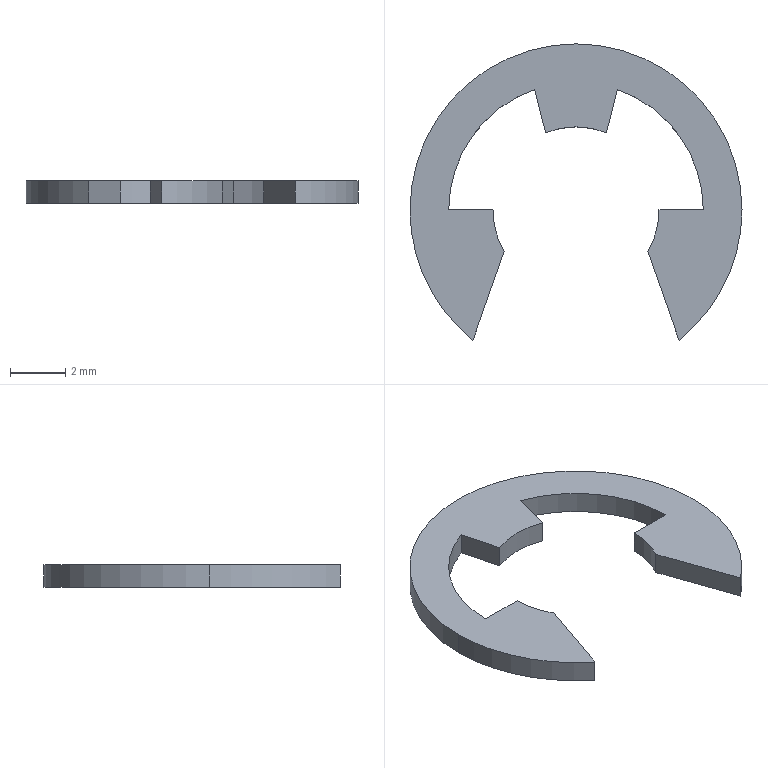Part | STEP file | 0246_016_NETWS6 | 1 solid | 16 faces | box 12 x 10.705 x 0.8 mm | volume 38.915 mm3 | cylinder 8 | plane 8 | commonest cylinder face diameters 6 x3 12 x3 9.2 x2
STEP:
#1=CARTESIAN_POINT('',(0.,0.,0.));
#2=DIRECTION('',(0.,0.,1.));
#3=DIRECTION('',(1.,0.,0.));
#4=AXIS2_PLACEMENT_3D('',#1,#2,#3);
#5=CARTESIAN_POINT('',(6.,0.,-0.4));
#6=VERTEX_POINT('',#5);
#7=CARTESIAN_POINT('',(-6.,0.,-0.4));
#8=VERTEX_POINT('',#7);
#9=CARTESIAN_POINT('',(0.,0.,-0.4));
#10=DIRECTION('',(0.,0.,1.));
#11=DIRECTION('',(1.,0.,0.));
#12=AXIS2_PLACEMENT_3D('',#9,#10,#11);
#13=CIRCLE('',#12,6.);
#14=CARTESIAN_POINT('',(0.,0.,0.4));
#15=DIRECTION('',(0.,0.,1.));
#16=DIRECTION('',(1.,0.,0.));
#17=AXIS2_PLACEMENT_3D('',#14,#15,#16);
#18=CYLINDRICAL_SURFACE('',#17,6.);
#19=CARTESIAN_POINT('',(0.,-0.8));
#20=DIRECTION('',(1.,0.));
#21=VECTOR('',#20,1.);
#22=LINE('',#19,#21);
#23=(GEOMETRIC_REPRESENTATION_CONTEXT(2)PARAMETRIC_REPRESENTATION_CONTEXT()REPRESENTATION_CONTEXT('',''));
#24=DEFINITIONAL_REPRESENTATION('',(#22),#23);
#25=PCURVE('',#18,#24);
#26=CARTESIAN_POINT('',(0.,0.,-0.4));
#27=DIRECTION('',(0.,0.,1.));
#28=DIRECTION('',(1.,0.,0.));
#29=AXIS2_PLACEMENT_3D('',#26,#27,#28);
#30=PLANE('',#29);
#31=CARTESIAN_POINT('',(0.,0.));
#32=DIRECTION('',(1.,0.));
#33=AXIS2_PLACEMENT_2D('',#31,#32);
#34=CIRCLE('',#33,6.);
#35=(GEOMETRIC_REPRESENTATION_CONTEXT(2)PARAMETRIC_REPRESENTATION_CONTEXT()REPRESENTATION_CONTEXT('',''));
#36=DEFINITIONAL_REPRESENTATION('',(#34),#35);
#37=PCURVE('',#30,#36);
#38=SURFACE_CURVE('',#13,(#25,#37),.PCURVE_S1.);
#39=EDGE_CURVE('',#6,#8,#38,.T.);
#40=ORIENTED_EDGE('',*,*,#39,.T.);
#41=CARTESIAN_POINT('',(-6.,0.,0.4));
#42=VERTEX_POINT('',#41);
#43=CARTESIAN_POINT('',(-6.,0.,0.4));
#44=DIRECTION('',(0.,0.,1.));
#45=VECTOR('',#44,1.);
#46=LINE('',#43,#45);
#47=CARTESIAN_POINT('',(3.142,0.));
#48=DIRECTION('',(0.,1.));
#49=VECTOR('',#48,1.);
#50=LINE('',#47,#49);
#51=(GEOMETRIC_REPRESENTATION_CONTEXT(2)PARAMETRIC_REPRESENTATION_CONTEXT()REPRESENTATION_CONTEXT('',''));
#52=DEFINITIONAL_REPRESENTATION('',(#50),#51);
#53=PCURVE('',#18,#52);
#54=CARTESIAN_POINT('',(0.,0.,0.4));
#55=DIRECTION('',(0.,0.,1.));
#56=DIRECTION('',(1.,0.,0.));
#57=AXIS2_PLACEMENT_3D('',#54,#55,#56);
#58=CYLINDRICAL_SURFACE('',#57,6.);
#59=CARTESIAN_POINT('',(3.142,0.));
#60=DIRECTION('',(0.,1.));
#61=VECTOR('',#60,1.);
#62=LINE('',#59,#61);
#63=(GEOMETRIC_REPRESENTATION_CONTEXT(2)PARAMETRIC_REPRESENTATION_CONTEXT()REPRESENTATION_CONTEXT('',''));
#64=DEFINITIONAL_REPRESENTATION('',(#62),#63);
#65=PCURVE('',#58,#64);
#66=SURFACE_CURVE('',#46,(#53,#65),.PCURVE_S1.);
#67=EDGE_CURVE('',#8,#42,#66,.T.);
#68=ORIENTED_EDGE('',*,*,#67,.T.);
#69=CARTESIAN_POINT('',(6.,0.,0.4));
#70=VERTEX_POINT('',#69);
#71=CARTESIAN_POINT('',(0.,0.,0.4));
#72=DIRECTION('',(0.,0.,-1.));
#73=DIRECTION('',(1.,0.,0.));
#74=AXIS2_PLACEMENT_3D('',#71,#72,#73);
#75=CIRCLE('',#74,6.);
#76=CARTESIAN_POINT('',(6.283,0.));
#77=DIRECTION('',(-1.,0.));
#78=VECTOR('',#77,1.);
#79=LINE('',#76,#78);
#80=(GEOMETRIC_REPRESENTATION_CONTEXT(2)PARAMETRIC_REPRESENTATION_CONTEXT()REPRESENTATION_CONTEXT('',''));
#81=DEFINITIONAL_REPRESENTATION('',(#79),#80);
#82=PCURVE('',#18,#81);
#83=CARTESIAN_POINT('',(0.,0.,0.4));
#84=DIRECTION('',(0.,0.,1.));
#85=DIRECTION('',(1.,0.,0.));
#86=AXIS2_PLACEMENT_3D('',#83,#84,#85);
#87=PLANE('',#86);
#88=CARTESIAN_POINT('',(6.,0.));
#89=CARTESIAN_POINT('',(6.,-10.392));
#90=CARTESIAN_POINT('',(-3.,-5.196));
#91=CARTESIAN_POINT('',(-12.,0.));
#92=CARTESIAN_POINT('',(-3.,5.196));
#93=CARTESIAN_POINT('',(6.,10.392));
#94=CARTESIAN_POINT('',(6.,0.));
#95=(BOUNDED_CURVE()B_SPLINE_CURVE(2,(#88,#89,#90,#91,#92,#93,#94),.UNSPECIFIED.,.T.,.F.)B_SPLINE_CURVE_WITH_KNOTS((1,2,2,2,2,1),(-2.094,0.,2.094,4.189,6.283,8.378),.UNSPECIFIED.)CURVE()GEOMETRIC_REPRESENTATION_ITEM()RATIONAL_B_SPLINE_CURVE((1.,0.5,1.,0.5,1.,0.5,1.))REPRESENTATION_ITEM(''));
#96=(GEOMETRIC_REPRESENTATION_CONTEXT(2)PARAMETRIC_REPRESENTATION_CONTEXT()REPRESENTATION_CONTEXT('',''));
#97=DEFINITIONAL_REPRESENTATION('',(#95),#96);
#98=PCURVE('',#87,#97);
#99=SURFACE_CURVE('',#75,(#82,#98),.PCURVE_S1.);
#100=EDGE_CURVE('',#42,#70,#99,.T.);
#101=ORIENTED_EDGE('',*,*,#100,.T.);
#102=CARTESIAN_POINT('',(6.,0.,0.4));
#103=DIRECTION('',(0.,0.,1.));
#104=VECTOR('',#103,1.);
#105=LINE('',#102,#104);
#106=CARTESIAN_POINT('',(0.,0.));
#107=DIRECTION('',(0.,1.));
#108=VECTOR('',#107,1.);
#109=LINE('',#106,#108);
#110=(GEOMETRIC_REPRESENTATION_CONTEXT(2)PARAMETRIC_REPRESENTATION_CONTEXT()REPRESENTATION_CONTEXT('',''));
#111=DEFINITIONAL_REPRESENTATION('',(#109),#110);
#112=PCURVE('',#18,#111);
#113=CARTESIAN_POINT('',(0.,0.,0.4));
#114=DIRECTION('',(0.,0.,1.));
#115=DIRECTION('',(1.,0.,0.));
#116=AXIS2_PLACEMENT_3D('',#113,#114,#115);
#117=CYLINDRICAL_SURFACE('',#116,6.);
#118=CARTESIAN_POINT('',(6.283,0.));
#119=DIRECTION('',(0.,1.));
#120=VECTOR('',#119,1.);
#121=LINE('',#118,#120);
#122=(GEOMETRIC_REPRESENTATION_CONTEXT(2)PARAMETRIC_REPRESENTATION_CONTEXT()REPRESENTATION_CONTEXT('',''));
#123=DEFINITIONAL_REPRESENTATION('',(#121),#122);
#124=PCURVE('',#117,#123);
#125=SURFACE_CURVE('',#105,(#112,#124),.PCURVE_S1.);
#126=EDGE_CURVE('',#6,#70,#125,.T.);
#127=ORIENTED_EDGE('',*,*,#126,.F.);
#128=EDGE_LOOP('',(#40,#68,#101,#127));
#129=FACE_BOUND('',#128,.T.);
#130=ADVANCED_FACE('',(#129),#18,.T.);
#131=CARTESIAN_POINT('',(3.723,-4.705,-0.4));
#132=VERTEX_POINT('',#131);
#133=CARTESIAN_POINT('',(0.,0.,-0.4));
#134=DIRECTION('',(0.,0.,1.));
#135=DIRECTION('',(1.,0.,0.));
#136=AXIS2_PLACEMENT_3D('',#133,#134,#135);
#137=CIRCLE('',#136,6.);
#138=CARTESIAN_POINT('',(0.,-0.8));
#139=DIRECTION('',(1.,0.));
#140=VECTOR('',#139,1.);
#141=LINE('',#138,#140);
#142=(GEOMETRIC_REPRESENTATION_CONTEXT(2)PARAMETRIC_REPRESENTATION_CONTEXT()REPRESENTATION_CONTEXT('',''));
#143=DEFINITIONAL_REPRESENTATION('',(#141),#142);
#144=PCURVE('',#117,#143);
#145=CARTESIAN_POINT('',(0.,0.));
#146=DIRECTION('',(1.,0.));
#147=AXIS2_PLACEMENT_2D('',#145,#146);
#148=CIRCLE('',#147,6.);
#149=(GEOMETRIC_REPRESENTATION_CONTEXT(2)PARAMETRIC_REPRESENTATION_CONTEXT()REPRESENTATION_CONTEXT('',''));
#150=DEFINITIONAL_REPRESENTATION('',(#148),#149);
#151=PCURVE('',#30,#150);
#152=SURFACE_CURVE('',#137,(#144,#151),.PCURVE_S1.);
#153=EDGE_CURVE('',#132,#6,#152,.T.);
#154=ORIENTED_EDGE('',*,*,#153,.T.);
#155=ORIENTED_EDGE('',*,*,#126,.T.);
#156=CARTESIAN_POINT('',(3.723,-4.705,0.4));
#157=VERTEX_POINT('',#156);
#158=CARTESIAN_POINT('',(0.,0.,0.4));
#159=DIRECTION('',(0.,0.,-1.));
#160=DIRECTION('',(1.,0.,0.));
#161=AXIS2_PLACEMENT_3D('',#158,#159,#160);
#162=CIRCLE('',#161,6.);
#163=CARTESIAN_POINT('',(6.283,0.));
#164=DIRECTION('',(-1.,0.));
#165=VECTOR('',#164,1.);
#166=LINE('',#163,#165);
#167=(GEOMETRIC_REPRESENTATION_CONTEXT(2)PARAMETRIC_REPRESENTATION_CONTEXT()REPRESENTATION_CONTEXT('',''));
#168=DEFINITIONAL_REPRESENTATION('',(#166),#167);
#169=PCURVE('',#117,#168);
#170=CARTESIAN_POINT('',(6.,0.));
#171=CARTESIAN_POINT('',(6.,-10.392));
#172=CARTESIAN_POINT('',(-3.,-5.196));
#173=CARTESIAN_POINT('',(-12.,0.));
#174=CARTESIAN_POINT('',(-3.,5.196));
#175=CARTESIAN_POINT('',(6.,10.392));
#176=CARTESIAN_POINT('',(6.,0.));
#177=(BOUNDED_CURVE()B_SPLINE_CURVE(2,(#170,#171,#172,#173,#174,#175,#176),.UNSPECIFIED.,.T.,.F.)B_SPLINE_CURVE_WITH_KNOTS((1,2,2,2,2,1),(-2.094,0.,2.094,4.189,6.283,8.378),.UNSPECIFIED.)CURVE()GEOMETRIC_REPRESENTATION_ITEM()RATIONAL_B_SPLINE_CURVE((1.,0.5,1.,0.5,1.,0.5,1.))REPRESENTATION_ITEM(''));
#178=(GEOMETRIC_REPRESENTATION_CONTEXT(2)PARAMETRIC_REPRESENTATION_CONTEXT()REPRESENTATION_CONTEXT('',''));
#179=DEFINITIONAL_REPRESENTATION('',(#177),#178);
#180=PCURVE('',#87,#179);
#181=SURFACE_CURVE('',#162,(#169,#180),.PCURVE_S1.);
#182=EDGE_CURVE('',#70,#157,#181,.T.);
#183=ORIENTED_EDGE('',*,*,#182,.T.);
#184=CARTESIAN_POINT('',(3.723,-4.705,0.4));
#185=DIRECTION('',(0.,0.,-1.));
#186=VECTOR('',#185,1.);
#187=LINE('',#184,#186);
#188=CARTESIAN_POINT('',(5.382,0.));
#189=DIRECTION('',(0.,-1.));
#190=VECTOR('',#189,1.);
#191=LINE('',#188,#190);
#192=(GEOMETRIC_REPRESENTATION_CONTEXT(2)PARAMETRIC_REPRESENTATION_CONTEXT()REPRESENTATION_CONTEXT('',''));
#193=DEFINITIONAL_REPRESENTATION('',(#191),#192);
#194=PCURVE('',#117,#193);
#195=CARTESIAN_POINT('',(2.6,-1.497,0.4));
#196=DIRECTION('',(-0.9438,-0.3305,0.));
#197=DIRECTION('',(0.3305,-0.9438,0.));
#198=AXIS2_PLACEMENT_3D('',#195,#196,#197);
#199=PLANE('',#198);
#200=CARTESIAN_POINT('',(3.399,0.));
#201=DIRECTION('',(0.,-1.));
#202=VECTOR('',#201,1.);
#203=LINE('',#200,#202);
#204=(GEOMETRIC_REPRESENTATION_CONTEXT(2)PARAMETRIC_REPRESENTATION_CONTEXT()REPRESENTATION_CONTEXT('',''));
#205=DEFINITIONAL_REPRESENTATION('',(#203),#204);
#206=PCURVE('',#199,#205);
#207=SURFACE_CURVE('',#187,(#194,#206),.PCURVE_S1.);
#208=EDGE_CURVE('',#157,#132,#207,.T.);
#209=ORIENTED_EDGE('',*,*,#208,.T.);
#210=EDGE_LOOP('',(#154,#155,#183,#209));
#211=FACE_BOUND('',#210,.T.);
#212=ADVANCED_FACE('',(#211),#117,.T.);
#213=CARTESIAN_POINT('',(-3.723,-4.705,-0.4));
#214=VERTEX_POINT('',#213);
#215=CARTESIAN_POINT('',(-2.6,-1.497,-0.4));
#216=VERTEX_POINT('',#215);
#217=CARTESIAN_POINT('',(-3.723,-4.705,-0.4));
#218=DIRECTION('',(0.3305,0.9438,0.));
#219=VECTOR('',#218,1.);
#220=LINE('',#217,#219);
#221=CARTESIAN_POINT('',(-3.723,-4.705));
#222=DIRECTION('',(0.3305,0.9438));
#223=VECTOR('',#222,1.);
#224=LINE('',#221,#223);
#225=(GEOMETRIC_REPRESENTATION_CONTEXT(2)PARAMETRIC_REPRESENTATION_CONTEXT()REPRESENTATION_CONTEXT('',''));
#226=DEFINITIONAL_REPRESENTATION('',(#224),#225);
#227=PCURVE('',#30,#226);
#228=CARTESIAN_POINT('',(-3.723,-4.705,0.4));
#229=DIRECTION('',(0.9438,-0.3305,0.));
#230=DIRECTION('',(0.3305,0.9438,0.));
#231=AXIS2_PLACEMENT_3D('',#228,#229,#230);
#232=PLANE('',#231);
#233=CARTESIAN_POINT('',(0.,-0.8));
#234=DIRECTION('',(1.,0.));
#235=VECTOR('',#234,1.);
#236=LINE('',#233,#235);
#237=(GEOMETRIC_REPRESENTATION_CONTEXT(2)PARAMETRIC_REPRESENTATION_CONTEXT()REPRESENTATION_CONTEXT('',''));
#238=DEFINITIONAL_REPRESENTATION('',(#236),#237);
#239=PCURVE('',#232,#238);
#240=SURFACE_CURVE('',#220,(#227,#239),.PCURVE_S1.);
#241=EDGE_CURVE('',#214,#216,#240,.T.);
#242=ORIENTED_EDGE('',*,*,#241,.F.);
#243=CARTESIAN_POINT('',(0.,0.,-0.4));
#244=DIRECTION('',(0.,0.,1.));
#245=DIRECTION('',(1.,0.,0.));
#246=AXIS2_PLACEMENT_3D('',#243,#244,#245);
#247=CIRCLE('',#246,6.);
#248=CARTESIAN_POINT('',(0.,0.));
#249=DIRECTION('',(1.,0.));
#250=AXIS2_PLACEMENT_2D('',#248,#249);
#251=CIRCLE('',#250,6.);
#252=(GEOMETRIC_REPRESENTATION_CONTEXT(2)PARAMETRIC_REPRESENTATION_CONTEXT()REPRESENTATION_CONTEXT('',''));
#253=DEFINITIONAL_REPRESENTATION('',(#251),#252);
#254=PCURVE('',#30,#253);
#255=CARTESIAN_POINT('',(0.,-0.8));
#256=DIRECTION('',(1.,0.));
#257=VECTOR('',#256,1.);
#258=LINE('',#255,#257);
#259=(GEOMETRIC_REPRESENTATION_CONTEXT(2)PARAMETRIC_REPRESENTATION_CONTEXT()REPRESENTATION_CONTEXT('',''));
#260=DEFINITIONAL_REPRESENTATION('',(#258),#259);
#261=PCURVE('',#58,#260);
#262=SURFACE_CURVE('',#247,(#254,#261),.PCURVE_S1.);
#263=EDGE_CURVE('',#8,#214,#262,.T.);
#264=ORIENTED_EDGE('',*,*,#263,.F.);
#265=ORIENTED_EDGE('',*,*,#39,.F.);
#266=ORIENTED_EDGE('',*,*,#153,.F.);
#267=CARTESIAN_POINT('',(2.6,-1.497,-0.4));
#268=VERTEX_POINT('',#267);
#269=CARTESIAN_POINT('',(2.6,-1.497,-0.4));
#270=DIRECTION('',(0.3305,-0.9438,0.));
#271=VECTOR('',#270,1.);
#272=LINE('',#269,#271);
#273=CARTESIAN_POINT('',(2.6,-1.497));
#274=DIRECTION('',(0.3305,-0.9438));
#275=VECTOR('',#274,1.);
#276=LINE('',#273,#275);
#277=(GEOMETRIC_REPRESENTATION_CONTEXT(2)PARAMETRIC_REPRESENTATION_CONTEXT()REPRESENTATION_CONTEXT('',''));
#278=DEFINITIONAL_REPRESENTATION('',(#276),#277);
#279=PCURVE('',#30,#278);
#280=CARTESIAN_POINT('',(0.,-0.8));
#281=DIRECTION('',(1.,0.));
#282=VECTOR('',#281,1.);
#283=LINE('',#280,#282);
#284=(GEOMETRIC_REPRESENTATION_CONTEXT(2)PARAMETRIC_REPRESENTATION_CONTEXT()REPRESENTATION_CONTEXT('',''));
#285=DEFINITIONAL_REPRESENTATION('',(#283),#284);
#286=PCURVE('',#199,#285);
#287=SURFACE_CURVE('',#272,(#279,#286),.PCURVE_S1.);
#288=EDGE_CURVE('',#268,#132,#287,.T.);
#289=ORIENTED_EDGE('',*,*,#288,.F.);
#290=CARTESIAN_POINT('',(3.,0.,-0.4));
#291=VERTEX_POINT('',#290);
#292=CARTESIAN_POINT('',(0.,0.,-0.4));
#293=DIRECTION('',(0.,0.,-1.));
#294=DIRECTION('',(1.,0.,0.));
#295=AXIS2_PLACEMENT_3D('',#292,#293,#294);
#296=CIRCLE('',#295,3.);
#297=CARTESIAN_POINT('',(3.,0.));
#298=CARTESIAN_POINT('',(3.,-5.196));
#299=CARTESIAN_POINT('',(-1.5,-2.598));
#300=CARTESIAN_POINT('',(-6.,0.));
#301=CARTESIAN_POINT('',(-1.5,2.598));
#302=CARTESIAN_POINT('',(3.,5.196));
#303=CARTESIAN_POINT('',(3.,0.));
#304=(BOUNDED_CURVE()B_SPLINE_CURVE(2,(#297,#298,#299,#300,#301,#302,#303),.UNSPECIFIED.,.T.,.F.)B_SPLINE_CURVE_WITH_KNOTS((1,2,2,2,2,1),(-2.094,0.,2.094,4.189,6.283,8.378),.UNSPECIFIED.)CURVE()GEOMETRIC_REPRESENTATION_ITEM()RATIONAL_B_SPLINE_CURVE((1.,0.5,1.,0.5,1.,0.5,1.))REPRESENTATION_ITEM(''));
#305=(GEOMETRIC_REPRESENTATION_CONTEXT(2)PARAMETRIC_REPRESENTATION_CONTEXT()REPRESENTATION_CONTEXT('',''));
#306=DEFINITIONAL_REPRESENTATION('',(#304),#305);
#307=PCURVE('',#30,#306);
#308=CARTESIAN_POINT('',(0.,0.,0.4));
#309=DIRECTION('',(0.,0.,1.));
#310=DIRECTION('',(1.,0.,0.));
#311=AXIS2_PLACEMENT_3D('',#308,#309,#310);
#312=CYLINDRICAL_SURFACE('',#311,3.);
#313=CARTESIAN_POINT('',(6.283,-0.8));
#314=DIRECTION('',(-1.,0.));
#315=VECTOR('',#314,1.);
#316=LINE('',#313,#315);
#317=(GEOMETRIC_REPRESENTATION_CONTEXT(2)PARAMETRIC_REPRESENTATION_CONTEXT()REPRESENTATION_CONTEXT('',''));
#318=DEFINITIONAL_REPRESENTATION('',(#316),#317);
#319=PCURVE('',#312,#318);
#320=SURFACE_CURVE('',#296,(#307,#319),.PCURVE_S1.);
#321=EDGE_CURVE('',#291,#268,#320,.T.);
#322=ORIENTED_EDGE('',*,*,#321,.F.);
#323=CARTESIAN_POINT('',(4.6,0.,-0.4));
#324=VERTEX_POINT('',#323);
#325=CARTESIAN_POINT('',(0.,0.,-0.4));
#326=DIRECTION('',(-1.,0.,0.));
#327=VECTOR('',#326,1.);
#328=LINE('',#325,#327);
#329=CARTESIAN_POINT('',(0.,0.));
#330=DIRECTION('',(-1.,0.));
#331=VECTOR('',#330,1.);
#332=LINE('',#329,#331);
#333=(GEOMETRIC_REPRESENTATION_CONTEXT(2)PARAMETRIC_REPRESENTATION_CONTEXT()REPRESENTATION_CONTEXT('',''));
#334=DEFINITIONAL_REPRESENTATION('',(#332),#333);
#335=PCURVE('',#30,#334);
#336=CARTESIAN_POINT('',(4.6,0.,0.4));
#337=DIRECTION('',(0.,1.,0.));
#338=DIRECTION('',(0.,0.,1.));
#339=AXIS2_PLACEMENT_3D('',#336,#337,#338);
#340=PLANE('',#339);
#341=CARTESIAN_POINT('',(-0.8,-4.6));
#342=DIRECTION('',(0.,-1.));
#343=VECTOR('',#342,1.);
#344=LINE('',#341,#343);
#345=(GEOMETRIC_REPRESENTATION_CONTEXT(2)PARAMETRIC_REPRESENTATION_CONTEXT()REPRESENTATION_CONTEXT('',''));
#346=DEFINITIONAL_REPRESENTATION('',(#344),#345);
#347=PCURVE('',#340,#346);
#348=SURFACE_CURVE('',#328,(#335,#347),.PCURVE_S1.);
#349=EDGE_CURVE('',#324,#291,#348,.T.);
#350=ORIENTED_EDGE('',*,*,#349,.F.);
#351=CARTESIAN_POINT('',(1.5,4.349,-0.4));
#352=VERTEX_POINT('',#351);
#353=CARTESIAN_POINT('',(0.,0.,-0.4));
#354=DIRECTION('',(0.,0.,-1.));
#355=DIRECTION('',(1.,0.,0.));
#356=AXIS2_PLACEMENT_3D('',#353,#354,#355);
#357=CIRCLE('',#356,4.6);
#358=CARTESIAN_POINT('',(4.6,0.));
#359=CARTESIAN_POINT('',(4.6,-7.967));
#360=CARTESIAN_POINT('',(-2.3,-3.984));
#361=CARTESIAN_POINT('',(-9.2,0.));
#362=CARTESIAN_POINT('',(-2.3,3.984));
#363=CARTESIAN_POINT('',(4.6,7.967));
#364=CARTESIAN_POINT('',(4.6,0.));
#365=(BOUNDED_CURVE()B_SPLINE_CURVE(2,(#358,#359,#360,#361,#362,#363,#364),.UNSPECIFIED.,.T.,.F.)B_SPLINE_CURVE_WITH_KNOTS((1,2,2,2,2,1),(-2.094,0.,2.094,4.189,6.283,8.378),.UNSPECIFIED.)CURVE()GEOMETRIC_REPRESENTATION_ITEM()RATIONAL_B_SPLINE_CURVE((1.,0.5,1.,0.5,1.,0.5,1.))REPRESENTATION_ITEM(''));
#366=(GEOMETRIC_REPRESENTATION_CONTEXT(2)PARAMETRIC_REPRESENTATION_CONTEXT()REPRESENTATION_CONTEXT('',''));
#367=DEFINITIONAL_REPRESENTATION('',(#365),#366);
#368=PCURVE('',#30,#367);
#369=CARTESIAN_POINT('',(0.,0.,0.4));
#370=DIRECTION('',(0.,0.,1.));
#371=DIRECTION('',(1.,0.,0.));
#372=AXIS2_PLACEMENT_3D('',#369,#370,#371);
#373=CYLINDRICAL_SURFACE('',#372,4.6);
#374=CARTESIAN_POINT('',(6.283,-0.8));
#375=DIRECTION('',(-1.,0.));
#376=VECTOR('',#375,1.);
#377=LINE('',#374,#376);
#378=(GEOMETRIC_REPRESENTATION_CONTEXT(2)PARAMETRIC_REPRESENTATION_CONTEXT()REPRESENTATION_CONTEXT('',''));
#379=DEFINITIONAL_REPRESENTATION('',(#377),#378);
#380=PCURVE('',#373,#379);
#381=SURFACE_CURVE('',#357,(#368,#380),.PCURVE_S1.);
#382=EDGE_CURVE('',#352,#324,#381,.T.);
#383=ORIENTED_EDGE('',*,*,#382,.F.);
#384=CARTESIAN_POINT('',(1.1,2.791,-0.4));
#385=VERTEX_POINT('',#384);
#386=CARTESIAN_POINT('',(1.1,2.791,-0.4));
#387=DIRECTION('',(0.2487,0.9686,0.));
#388=VECTOR('',#387,1.);
#389=LINE('',#386,#388);
#390=CARTESIAN_POINT('',(1.1,2.791));
#391=DIRECTION('',(0.2487,0.9686));
#392=VECTOR('',#391,1.);
#393=LINE('',#390,#392);
#394=(GEOMETRIC_REPRESENTATION_CONTEXT(2)PARAMETRIC_REPRESENTATION_CONTEXT()REPRESENTATION_CONTEXT('',''));
#395=DEFINITIONAL_REPRESENTATION('',(#393),#394);
#396=PCURVE('',#30,#395);
#397=CARTESIAN_POINT('',(1.1,2.791,0.4));
#398=DIRECTION('',(0.9686,-0.2487,0.));
#399=DIRECTION('',(0.2487,0.9686,0.));
#400=AXIS2_PLACEMENT_3D('',#397,#398,#399);
#401=PLANE('',#400);
#402=CARTESIAN_POINT('',(0.,-0.8));
#403=DIRECTION('',(1.,0.));
#404=VECTOR('',#403,1.);
#405=LINE('',#402,#404);
#406=(GEOMETRIC_REPRESENTATION_CONTEXT(2)PARAMETRIC_REPRESENTATION_CONTEXT()REPRESENTATION_CONTEXT('',''));
#407=DEFINITIONAL_REPRESENTATION('',(#405),#406);
#408=PCURVE('',#401,#407);
#409=SURFACE_CURVE('',#389,(#396,#408),.PCURVE_S1.);
#410=EDGE_CURVE('',#385,#352,#409,.T.);
#411=ORIENTED_EDGE('',*,*,#410,.F.);
#412=CARTESIAN_POINT('',(-1.1,2.791,-0.4));
#413=VERTEX_POINT('',#412);
#414=CARTESIAN_POINT('',(0.,0.,-0.4));
#415=DIRECTION('',(0.,0.,-1.));
#416=DIRECTION('',(1.,0.,0.));
#417=AXIS2_PLACEMENT_3D('',#414,#415,#416);
#418=CIRCLE('',#417,3.);
#419=CARTESIAN_POINT('',(3.,0.));
#420=CARTESIAN_POINT('',(3.,-5.196));
#421=CARTESIAN_POINT('',(-1.5,-2.598));
#422=CARTESIAN_POINT('',(-6.,0.));
#423=CARTESIAN_POINT('',(-1.5,2.598));
#424=CARTESIAN_POINT('',(3.,5.196));
#425=CARTESIAN_POINT('',(3.,0.));
#426=(BOUNDED_CURVE()B_SPLINE_CURVE(2,(#419,#420,#421,#422,#423,#424,#425),.UNSPECIFIED.,.T.,.F.)B_SPLINE_CURVE_WITH_KNOTS((1,2,2,2,2,1),(-2.094,0.,2.094,4.189,6.283,8.378),.UNSPECIFIED.)CURVE()GEOMETRIC_REPRESENTATION_ITEM()RATIONAL_B_SPLINE_CURVE((1.,0.5,1.,0.5,1.,0.5,1.))REPRESENTATION_ITEM(''));
#427=(GEOMETRIC_REPRESENTATION_CONTEXT(2)PARAMETRIC_REPRESENTATION_CONTEXT()REPRESENTATION_CONTEXT('',''));
#428=DEFINITIONAL_REPRESENTATION('',(#426),#427);
#429=PCURVE('',#30,#428);
#430=CARTESIAN_POINT('',(0.,0.,0.4));
#431=DIRECTION('',(0.,0.,1.));
#432=DIRECTION('',(1.,0.,0.));
#433=AXIS2_PLACEMENT_3D('',#430,#431,#432);
#434=CYLINDRICAL_SURFACE('',#433,3.);
#435=CARTESIAN_POINT('',(6.283,-0.8));
#436=DIRECTION('',(-1.,0.));
#437=VECTOR('',#436,1.);
#438=LINE('',#435,#437);
#439=(GEOMETRIC_REPRESENTATION_CONTEXT(2)PARAMETRIC_REPRESENTATION_CONTEXT()REPRESENTATION_CONTEXT('',''));
#440=DEFINITIONAL_REPRESENTATION('',(#438),#439);
#441=PCURVE('',#434,#440);
#442=SURFACE_CURVE('',#418,(#429,#441),.PCURVE_S1.);
#443=EDGE_CURVE('',#413,#385,#442,.T.);
#444=ORIENTED_EDGE('',*,*,#443,.F.);
#445=CARTESIAN_POINT('',(-1.5,4.349,-0.4));
#446=VERTEX_POINT('',#445);
#447=CARTESIAN_POINT('',(-1.5,4.349,-0.4));
#448=DIRECTION('',(0.2487,-0.9686,0.));
#449=VECTOR('',#448,1.);
#450=LINE('',#447,#449);
#451=CARTESIAN_POINT('',(-1.5,4.349));
#452=DIRECTION('',(0.2487,-0.9686));
#453=VECTOR('',#452,1.);
#454=LINE('',#451,#453);
#455=(GEOMETRIC_REPRESENTATION_CONTEXT(2)PARAMETRIC_REPRESENTATION_CONTEXT()REPRESENTATION_CONTEXT('',''));
#456=DEFINITIONAL_REPRESENTATION('',(#454),#455);
#457=PCURVE('',#30,#456);
#458=CARTESIAN_POINT('',(-1.5,4.349,0.4));
#459=DIRECTION('',(-0.9686,-0.2487,0.));
#460=DIRECTION('',(0.2487,-0.9686,0.));
#461=AXIS2_PLACEMENT_3D('',#458,#459,#460);
#462=PLANE('',#461);
#463=CARTESIAN_POINT('',(0.,-0.8));
#464=DIRECTION('',(1.,0.));
#465=VECTOR('',#464,1.);
#466=LINE('',#463,#465);
#467=(GEOMETRIC_REPRESENTATION_CONTEXT(2)PARAMETRIC_REPRESENTATION_CONTEXT()REPRESENTATION_CONTEXT('',''));
#468=DEFINITIONAL_REPRESENTATION('',(#466),#467);
#469=PCURVE('',#462,#468);
#470=SURFACE_CURVE('',#450,(#457,#469),.PCURVE_S1.);
#471=EDGE_CURVE('',#446,#413,#470,.T.);
#472=ORIENTED_EDGE('',*,*,#471,.F.);
#473=CARTESIAN_POINT('',(-4.6,0.,-0.4));
#474=VERTEX_POINT('',#473);
#475=CARTESIAN_POINT('',(0.,0.,-0.4));
#476=DIRECTION('',(0.,0.,-1.));
#477=DIRECTION('',(1.,0.,0.));
#478=AXIS2_PLACEMENT_3D('',#475,#476,#477);
#479=CIRCLE('',#478,4.6);
#480=CARTESIAN_POINT('',(4.6,0.));
#481=CARTESIAN_POINT('',(4.6,-7.967));
#482=CARTESIAN_POINT('',(-2.3,-3.984));
#483=CARTESIAN_POINT('',(-9.2,0.));
#484=CARTESIAN_POINT('',(-2.3,3.984));
#485=CARTESIAN_POINT('',(4.6,7.967));
#486=CARTESIAN_POINT('',(4.6,0.));
#487=(BOUNDED_CURVE()B_SPLINE_CURVE(2,(#480,#481,#482,#483,#484,#485,#486),.UNSPECIFIED.,.T.,.F.)B_SPLINE_CURVE_WITH_KNOTS((1,2,2,2,2,1),(-2.094,0.,2.094,4.189,6.283,8.378),.UNSPECIFIED.)CURVE()GEOMETRIC_REPRESENTATION_ITEM()RATIONAL_B_SPLINE_CURVE((1.,0.5,1.,0.5,1.,0.5,1.))REPRESENTATION_ITEM(''));
#488=(GEOMETRIC_REPRESENTATION_CONTEXT(2)PARAMETRIC_REPRESENTATION_CONTEXT()REPRESENTATION_CONTEXT('',''));
#489=DEFINITIONAL_REPRESENTATION('',(#487),#488);
#490=PCURVE('',#30,#489);
#491=CARTESIAN_POINT('',(0.,0.,0.4));
#492=DIRECTION('',(0.,0.,1.));
#493=DIRECTION('',(1.,0.,0.));
#494=AXIS2_PLACEMENT_3D('',#491,#492,#493);
#495=CYLINDRICAL_SURFACE('',#494,4.6);
#496=CARTESIAN_POINT('',(6.283,-0.8));
#497=DIRECTION('',(-1.,0.));
#498=VECTOR('',#497,1.);
#499=LINE('',#496,#498);
#500=(GEOMETRIC_REPRESENTATION_CONTEXT(2)PARAMETRIC_REPRESENTATION_CONTEXT()REPRESENTATION_CONTEXT('',''));
#501=DEFINITIONAL_REPRESENTATION('',(#499),#500);
#502=PCURVE('',#495,#501);
#503=SURFACE_CURVE('',#479,(#490,#502),.PCURVE_S1.);
#504=EDGE_CURVE('',#474,#446,#503,.T.);
#505=ORIENTED_EDGE('',*,*,#504,.F.);
#506=CARTESIAN_POINT('',(-3.,0.,-0.4));
#507=VERTEX_POINT('',#506);
#508=CARTESIAN_POINT('',(0.,0.,-0.4));
#509=DIRECTION('',(-1.,0.,0.));
#510=VECTOR('',#509,1.);
#511=LINE('',#508,#510);
#512=CARTESIAN_POINT('',(0.,0.));
#513=DIRECTION('',(-1.,0.));
#514=VECTOR('',#513,1.);
#515=LINE('',#512,#514);
#516=(GEOMETRIC_REPRESENTATION_CONTEXT(2)PARAMETRIC_REPRESENTATION_CONTEXT()REPRESENTATION_CONTEXT('',''));
#517=DEFINITIONAL_REPRESENTATION('',(#515),#516);
#518=PCURVE('',#30,#517);
#519=CARTESIAN_POINT('',(-3.,0.,0.4));
#520=DIRECTION('',(0.,1.,0.));
#521=DIRECTION('',(0.,0.,1.));
#522=AXIS2_PLACEMENT_3D('',#519,#520,#521);
#523=PLANE('',#522);
#524=CARTESIAN_POINT('',(-0.8,3.));
#525=DIRECTION('',(0.,-1.));
#526=VECTOR('',#525,1.);
#527=LINE('',#524,#526);
#528=(GEOMETRIC_REPRESENTATION_CONTEXT(2)PARAMETRIC_REPRESENTATION_CONTEXT()REPRESENTATION_CONTEXT('',''));
#529=DEFINITIONAL_REPRESENTATION('',(#527),#528);
#530=PCURVE('',#523,#529);
#531=SURFACE_CURVE('',#511,(#518,#530),.PCURVE_S1.);
#532=EDGE_CURVE('',#507,#474,#531,.T.);
#533=ORIENTED_EDGE('',*,*,#532,.F.);
#534=CARTESIAN_POINT('',(0.,0.,-0.4));
#535=DIRECTION('',(0.,0.,-1.));
#536=DIRECTION('',(1.,0.,0.));
#537=AXIS2_PLACEMENT_3D('',#534,#535,#536);
#538=CIRCLE('',#537,3.);
#539=CARTESIAN_POINT('',(3.,0.));
#540=CARTESIAN_POINT('',(3.,-5.196));
#541=CARTESIAN_POINT('',(-1.5,-2.598));
#542=CARTESIAN_POINT('',(-6.,0.));
#543=CARTESIAN_POINT('',(-1.5,2.598));
#544=CARTESIAN_POINT('',(3.,5.196));
#545=CARTESIAN_POINT('',(3.,0.));
#546=(BOUNDED_CURVE()B_SPLINE_CURVE(2,(#539,#540,#541,#542,#543,#544,#545),.UNSPECIFIED.,.T.,.F.)B_SPLINE_CURVE_WITH_KNOTS((1,2,2,2,2,1),(-2.094,0.,2.094,4.189,6.283,8.378),.UNSPECIFIED.)CURVE()GEOMETRIC_REPRESENTATION_ITEM()RATIONAL_B_SPLINE_CURVE((1.,0.5,1.,0.5,1.,0.5,1.))REPRESENTATION_ITEM(''));
#547=(GEOMETRIC_REPRESENTATION_CONTEXT(2)PARAMETRIC_REPRESENTATION_CONTEXT()REPRESENTATION_CONTEXT('',''));
#548=DEFINITIONAL_REPRESENTATION('',(#546),#547);
#549=PCURVE('',#30,#548);
#550=CARTESIAN_POINT('',(0.,0.,0.4));
#551=DIRECTION('',(0.,0.,1.));
#552=DIRECTION('',(1.,0.,0.));
#553=AXIS2_PLACEMENT_3D('',#550,#551,#552);
#554=CYLINDRICAL_SURFACE('',#553,3.);
#555=CARTESIAN_POINT('',(6.283,-0.8));
#556=DIRECTION('',(-1.,0.));
#557=VECTOR('',#556,1.);
#558=LINE('',#555,#557);
#559=(GEOMETRIC_REPRESENTATION_CONTEXT(2)PARAMETRIC_REPRESENTATION_CONTEXT()REPRESENTATION_CONTEXT('',''));
#560=DEFINITIONAL_REPRESENTATION('',(#558),#559);
#561=PCURVE('',#554,#560);
#562=SURFACE_CURVE('',#538,(#549,#561),.PCURVE_S1.);
#563=EDGE_CURVE('',#216,#507,#562,.T.);
#564=ORIENTED_EDGE('',*,*,#563,.F.);
#565=EDGE_LOOP('',(#242,#264,#265,#266,#289,#322,#350,#383,#411,#444,#472,#505,#533,#564));
#566=FACE_BOUND('',#565,.T.);
#567=ADVANCED_FACE('',(#566),#30,.F.);
#568=CARTESIAN_POINT('',(-2.6,-1.497,0.4));
#569=VERTEX_POINT('',#568);
#570=CARTESIAN_POINT('',(-3.723,-4.705,0.4));
#571=VERTEX_POINT('',#570);
#572=CARTESIAN_POINT('',(-3.723,-4.705,0.4));
#573=DIRECTION('',(-0.3305,-0.9438,0.));
#574=VECTOR('',#573,1.);
#575=LINE('',#572,#574);
#576=CARTESIAN_POINT('',(0.,0.));
#577=DIRECTION('',(-1.,0.));
#578=VECTOR('',#577,1.);
#579=LINE('',#576,#578);
#580=(GEOMETRIC_REPRESENTATION_CONTEXT(2)PARAMETRIC_REPRESENTATION_CONTEXT()REPRESENTATION_CONTEXT('',''));
#581=DEFINITIONAL_REPRESENTATION('',(#579),#580);
#582=PCURVE('',#232,#581);
#583=CARTESIAN_POINT('',(-3.723,-4.705));
#584=DIRECTION('',(-0.3305,-0.9438));
#585=VECTOR('',#584,1.);
#586=LINE('',#583,#585);
#587=(GEOMETRIC_REPRESENTATION_CONTEXT(2)PARAMETRIC_REPRESENTATION_CONTEXT()REPRESENTATION_CONTEXT('',''));
#588=DEFINITIONAL_REPRESENTATION('',(#586),#587);
#589=PCURVE('',#87,#588);
#590=SURFACE_CURVE('',#575,(#582,#589),.PCURVE_S1.);
#591=EDGE_CURVE('',#569,#571,#590,.T.);
#592=ORIENTED_EDGE('',*,*,#591,.T.);
#593=CARTESIAN_POINT('',(-3.723,-4.705,0.4));
#594=DIRECTION('',(0.,0.,-1.));
#595=VECTOR('',#594,1.);
#596=LINE('',#593,#595);
#597=CARTESIAN_POINT('',(0.,0.));
#598=DIRECTION('',(0.,-1.));
#599=VECTOR('',#598,1.);
#600=LINE('',#597,#599);
#601=(GEOMETRIC_REPRESENTATION_CONTEXT(2)PARAMETRIC_REPRESENTATION_CONTEXT()REPRESENTATION_CONTEXT('',''));
#602=DEFINITIONAL_REPRESENTATION('',(#600),#601);
#603=PCURVE('',#232,#602);
#604=CARTESIAN_POINT('',(4.043,0.));
#605=DIRECTION('',(0.,-1.));
#606=VECTOR('',#605,1.);
#607=LINE('',#604,#606);
#608=(GEOMETRIC_REPRESENTATION_CONTEXT(2)PARAMETRIC_REPRESENTATION_CONTEXT()REPRESENTATION_CONTEXT('',''));
#609=DEFINITIONAL_REPRESENTATION('',(#607),#608);
#610=PCURVE('',#58,#609);
#611=SURFACE_CURVE('',#596,(#603,#610),.PCURVE_S1.);
#612=EDGE_CURVE('',#571,#214,#611,.T.);
#613=ORIENTED_EDGE('',*,*,#612,.T.);
#614=ORIENTED_EDGE('',*,*,#241,.T.);
#615=CARTESIAN_POINT('',(-2.6,-1.497,0.4));
#616=DIRECTION('',(0.,0.,1.));
#617=VECTOR('',#616,1.);
#618=LINE('',#615,#617);
#619=CARTESIAN_POINT('',(3.399,0.));
#620=DIRECTION('',(0.,1.));
#621=VECTOR('',#620,1.);
#622=LINE('',#619,#621);
#623=(GEOMETRIC_REPRESENTATION_CONTEXT(2)PARAMETRIC_REPRESENTATION_CONTEXT()REPRESENTATION_CONTEXT('',''));
#624=DEFINITIONAL_REPRESENTATION('',(#622),#623);
#625=PCURVE('',#232,#624);
#626=CARTESIAN_POINT('',(3.664,0.));
#627=DIRECTION('',(0.,1.));
#628=VECTOR('',#627,1.);
#629=LINE('',#626,#628);
#630=(GEOMETRIC_REPRESENTATION_CONTEXT(2)PARAMETRIC_REPRESENTATION_CONTEXT()REPRESENTATION_CONTEXT('',''));
#631=DEFINITIONAL_REPRESENTATION('',(#629),#630);
#632=PCURVE('',#554,#631);
#633=SURFACE_CURVE('',#618,(#625,#632),.PCURVE_S1.);
#634=EDGE_CURVE('',#216,#569,#633,.T.);
#635=ORIENTED_EDGE('',*,*,#634,.T.);
#636=EDGE_LOOP('',(#592,#613,#614,#635));
#637=FACE_BOUND('',#636,.T.);
#638=ADVANCED_FACE('',(#637),#232,.T.);
#639=ORIENTED_EDGE('',*,*,#67,.F.);
#640=ORIENTED_EDGE('',*,*,#263,.T.);
#641=ORIENTED_EDGE('',*,*,#612,.F.);
#642=CARTESIAN_POINT('',(0.,0.,0.4));
#643=DIRECTION('',(0.,0.,-1.));
#644=DIRECTION('',(1.,0.,0.));
#645=AXIS2_PLACEMENT_3D('',#642,#643,#644);
#646=CIRCLE('',#645,6.);
#647=CARTESIAN_POINT('',(6.283,0.));
#648=DIRECTION('',(-1.,0.));
#649=VECTOR('',#648,1.);
#650=LINE('',#647,#649);
#651=(GEOMETRIC_REPRESENTATION_CONTEXT(2)PARAMETRIC_REPRESENTATION_CONTEXT()REPRESENTATION_CONTEXT('',''));
#652=DEFINITIONAL_REPRESENTATION('',(#650),#651);
#653=PCURVE('',#58,#652);
#654=CARTESIAN_POINT('',(6.,0.));
#655=CARTESIAN_POINT('',(6.,-10.392));
#656=CARTESIAN_POINT('',(-3.,-5.196));
#657=CARTESIAN_POINT('',(-12.,0.));
#658=CARTESIAN_POINT('',(-3.,5.196));
#659=CARTESIAN_POINT('',(6.,10.392));
#660=CARTESIAN_POINT('',(6.,0.));
#661=(BOUNDED_CURVE()B_SPLINE_CURVE(2,(#654,#655,#656,#657,#658,#659,#660),.UNSPECIFIED.,.T.,.F.)B_SPLINE_CURVE_WITH_KNOTS((1,2,2,2,2,1),(-2.094,0.,2.094,4.189,6.283,8.378),.UNSPECIFIED.)CURVE()GEOMETRIC_REPRESENTATION_ITEM()RATIONAL_B_SPLINE_CURVE((1.,0.5,1.,0.5,1.,0.5,1.))REPRESENTATION_ITEM(''));
#662=(GEOMETRIC_REPRESENTATION_CONTEXT(2)PARAMETRIC_REPRESENTATION_CONTEXT()REPRESENTATION_CONTEXT('',''));
#663=DEFINITIONAL_REPRESENTATION('',(#661),#662);
#664=PCURVE('',#87,#663);
#665=SURFACE_CURVE('',#646,(#653,#664),.PCURVE_S1.);
#666=EDGE_CURVE('',#571,#42,#665,.T.);
#667=ORIENTED_EDGE('',*,*,#666,.T.);
#668=EDGE_LOOP('',(#639,#640,#641,#667));
#669=FACE_BOUND('',#668,.T.);
#670=ADVANCED_FACE('',(#669),#58,.T.);
#671=CARTESIAN_POINT('',(2.6,-1.497,0.4));
#672=VERTEX_POINT('',#671);
#673=CARTESIAN_POINT('',(2.6,-1.497,0.4));
#674=DIRECTION('',(-0.3305,0.9438,0.));
#675=VECTOR('',#674,1.);
#676=LINE('',#673,#675);
#677=CARTESIAN_POINT('',(0.,0.));
#678=DIRECTION('',(-1.,0.));
#679=VECTOR('',#678,1.);
#680=LINE('',#677,#679);
#681=(GEOMETRIC_REPRESENTATION_CONTEXT(2)PARAMETRIC_REPRESENTATION_CONTEXT()REPRESENTATION_CONTEXT('',''));
#682=DEFINITIONAL_REPRESENTATION('',(#680),#681);
#683=PCURVE('',#199,#682);
#684=CARTESIAN_POINT('',(2.6,-1.497));
#685=DIRECTION('',(-0.3305,0.9438));
#686=VECTOR('',#685,1.);
#687=LINE('',#684,#686);
#688=(GEOMETRIC_REPRESENTATION_CONTEXT(2)PARAMETRIC_REPRESENTATION_CONTEXT()REPRESENTATION_CONTEXT('',''));
#689=DEFINITIONAL_REPRESENTATION('',(#687),#688);
#690=PCURVE('',#87,#689);
#691=SURFACE_CURVE('',#676,(#683,#690),.PCURVE_S1.);
#692=EDGE_CURVE('',#157,#672,#691,.T.);
#693=ORIENTED_EDGE('',*,*,#692,.T.);
#694=CARTESIAN_POINT('',(2.6,-1.497,0.4));
#695=DIRECTION('',(0.,0.,-1.));
#696=VECTOR('',#695,1.);
#697=LINE('',#694,#696);
#698=CARTESIAN_POINT('',(0.,0.));
#699=DIRECTION('',(0.,-1.));
#700=VECTOR('',#699,1.);
#701=LINE('',#698,#700);
#702=(GEOMETRIC_REPRESENTATION_CONTEXT(2)PARAMETRIC_REPRESENTATION_CONTEXT()REPRESENTATION_CONTEXT('',''));
#703=DEFINITIONAL_REPRESENTATION('',(#701),#702);
#704=PCURVE('',#199,#703);
#705=CARTESIAN_POINT('',(5.761,0.));
#706=DIRECTION('',(0.,-1.));
#707=VECTOR('',#706,1.);
#708=LINE('',#705,#707);
#709=(GEOMETRIC_REPRESENTATION_CONTEXT(2)PARAMETRIC_REPRESENTATION_CONTEXT()REPRESENTATION_CONTEXT('',''));
#710=DEFINITIONAL_REPRESENTATION('',(#708),#709);
#711=PCURVE('',#312,#710);
#712=SURFACE_CURVE('',#697,(#704,#711),.PCURVE_S1.);
#713=EDGE_CURVE('',#672,#268,#712,.T.);
#714=ORIENTED_EDGE('',*,*,#713,.T.);
#715=ORIENTED_EDGE('',*,*,#288,.T.);
#716=ORIENTED_EDGE('',*,*,#208,.F.);
#717=EDGE_LOOP('',(#693,#714,#715,#716));
#718=FACE_BOUND('',#717,.T.);
#719=ADVANCED_FACE('',(#718),#199,.T.);
#720=ORIENTED_EDGE('',*,*,#321,.F.);
#721=CARTESIAN_POINT('',(3.,0.,0.4));
#722=VERTEX_POINT('',#721);
#723=CARTESIAN_POINT('',(3.,0.,0.4));
#724=DIRECTION('',(0.,0.,1.));
#725=VECTOR('',#724,1.);
#726=LINE('',#723,#725);
#727=CARTESIAN_POINT('',(6.283,0.));
#728=DIRECTION('',(0.,1.));
#729=VECTOR('',#728,1.);
#730=LINE('',#727,#729);
#731=(GEOMETRIC_REPRESENTATION_CONTEXT(2)PARAMETRIC_REPRESENTATION_CONTEXT()REPRESENTATION_CONTEXT('',''));
#732=DEFINITIONAL_REPRESENTATION('',(#730),#731);
#733=PCURVE('',#312,#732);
#734=CARTESIAN_POINT('',(0.,-1.6));
#735=DIRECTION('',(1.,0.));
#736=VECTOR('',#735,1.);
#737=LINE('',#734,#736);
#738=(GEOMETRIC_REPRESENTATION_CONTEXT(2)PARAMETRIC_REPRESENTATION_CONTEXT()REPRESENTATION_CONTEXT('',''));
#739=DEFINITIONAL_REPRESENTATION('',(#737),#738);
#740=PCURVE('',#340,#739);
#741=SURFACE_CURVE('',#726,(#733,#740),.PCURVE_S1.);
#742=EDGE_CURVE('',#291,#722,#741,.T.);
#743=ORIENTED_EDGE('',*,*,#742,.T.);
#744=CARTESIAN_POINT('',(0.,0.,0.4));
#745=DIRECTION('',(0.,0.,-1.));
#746=DIRECTION('',(1.,0.,0.));
#747=AXIS2_PLACEMENT_3D('',#744,#745,#746);
#748=CIRCLE('',#747,3.);
#749=CARTESIAN_POINT('',(6.283,0.));
#750=DIRECTION('',(-1.,0.));
#751=VECTOR('',#750,1.);
#752=LINE('',#749,#751);
#753=(GEOMETRIC_REPRESENTATION_CONTEXT(2)PARAMETRIC_REPRESENTATION_CONTEXT()REPRESENTATION_CONTEXT('',''));
#754=DEFINITIONAL_REPRESENTATION('',(#752),#753);
#755=PCURVE('',#312,#754);
#756=CARTESIAN_POINT('',(3.,0.));
#757=CARTESIAN_POINT('',(3.,-5.196));
#758=CARTESIAN_POINT('',(-1.5,-2.598));
#759=CARTESIAN_POINT('',(-6.,0.));
#760=CARTESIAN_POINT('',(-1.5,2.598));
#761=CARTESIAN_POINT('',(3.,5.196));
#762=CARTESIAN_POINT('',(3.,0.));
#763=(BOUNDED_CURVE()B_SPLINE_CURVE(2,(#756,#757,#758,#759,#760,#761,#762),.UNSPECIFIED.,.T.,.F.)B_SPLINE_CURVE_WITH_KNOTS((1,2,2,2,2,1),(-2.094,0.,2.094,4.189,6.283,8.378),.UNSPECIFIED.)CURVE()GEOMETRIC_REPRESENTATION_ITEM()RATIONAL_B_SPLINE_CURVE((1.,0.5,1.,0.5,1.,0.5,1.))REPRESENTATION_ITEM(''));
#764=(GEOMETRIC_REPRESENTATION_CONTEXT(2)PARAMETRIC_REPRESENTATION_CONTEXT()REPRESENTATION_CONTEXT('',''));
#765=DEFINITIONAL_REPRESENTATION('',(#763),#764);
#766=PCURVE('',#87,#765);
#767=SURFACE_CURVE('',#748,(#755,#766),.PCURVE_S1.);
#768=EDGE_CURVE('',#722,#672,#767,.T.);
#769=ORIENTED_EDGE('',*,*,#768,.T.);
#770=ORIENTED_EDGE('',*,*,#713,.T.);
#771=EDGE_LOOP('',(#720,#743,#769,#770));
#772=FACE_BOUND('',#771,.F.);
#773=ADVANCED_FACE('',(#772),#312,.F.);
#774=CARTESIAN_POINT('',(4.6,0.,0.4));
#775=VERTEX_POINT('',#774);
#776=CARTESIAN_POINT('',(4.6,0.,0.4));
#777=DIRECTION('',(1.,0.,0.));
#778=VECTOR('',#777,1.);
#779=LINE('',#776,#778);
#780=CARTESIAN_POINT('',(0.,0.));
#781=DIRECTION('',(0.,1.));
#782=VECTOR('',#781,1.);
#783=LINE('',#780,#782);
#784=(GEOMETRIC_REPRESENTATION_CONTEXT(2)PARAMETRIC_REPRESENTATION_CONTEXT()REPRESENTATION_CONTEXT('',''));
#785=DEFINITIONAL_REPRESENTATION('',(#783),#784);
#786=PCURVE('',#340,#785);
#787=CARTESIAN_POINT('',(4.6,0.));
#788=DIRECTION('',(1.,0.));
#789=VECTOR('',#788,1.);
#790=LINE('',#787,#789);
#791=(GEOMETRIC_REPRESENTATION_CONTEXT(2)PARAMETRIC_REPRESENTATION_CONTEXT()REPRESENTATION_CONTEXT('',''));
#792=DEFINITIONAL_REPRESENTATION('',(#790),#791);
#793=PCURVE('',#87,#792);
#794=SURFACE_CURVE('',#779,(#786,#793),.PCURVE_S1.);
#795=EDGE_CURVE('',#722,#775,#794,.T.);
#796=ORIENTED_EDGE('',*,*,#795,.T.);
#797=CARTESIAN_POINT('',(4.6,0.,0.4));
#798=DIRECTION('',(0.,0.,-1.));
#799=VECTOR('',#798,1.);
#800=LINE('',#797,#799);
#801=CARTESIAN_POINT('',(0.,0.));
#802=DIRECTION('',(-1.,0.));
#803=VECTOR('',#802,1.);
#804=LINE('',#801,#803);
#805=(GEOMETRIC_REPRESENTATION_CONTEXT(2)PARAMETRIC_REPRESENTATION_CONTEXT()REPRESENTATION_CONTEXT('',''));
#806=DEFINITIONAL_REPRESENTATION('',(#804),#805);
#807=PCURVE('',#340,#806);
#808=CARTESIAN_POINT('',(0.,0.));
#809=DIRECTION('',(0.,-1.));
#810=VECTOR('',#809,1.);
#811=LINE('',#808,#810);
#812=(GEOMETRIC_REPRESENTATION_CONTEXT(2)PARAMETRIC_REPRESENTATION_CONTEXT()REPRESENTATION_CONTEXT('',''));
#813=DEFINITIONAL_REPRESENTATION('',(#811),#812);
#814=PCURVE('',#373,#813);
#815=SURFACE_CURVE('',#800,(#807,#814),.PCURVE_S1.);
#816=EDGE_CURVE('',#775,#324,#815,.T.);
#817=ORIENTED_EDGE('',*,*,#816,.T.);
#818=ORIENTED_EDGE('',*,*,#349,.T.);
#819=ORIENTED_EDGE('',*,*,#742,.T.);
#820=EDGE_LOOP('',(#796,#817,#818,#819));
#821=FACE_BOUND('',#820,.T.);
#822=ADVANCED_FACE('',(#821),#340,.T.);
#823=ORIENTED_EDGE('',*,*,#382,.F.);
#824=CARTESIAN_POINT('',(1.5,4.349,0.4));
#825=VERTEX_POINT('',#824);
#826=CARTESIAN_POINT('',(1.5,4.349,0.4));
#827=DIRECTION('',(0.,0.,1.));
#828=VECTOR('',#827,1.);
#829=LINE('',#826,#828);
#830=CARTESIAN_POINT('',(1.239,0.));
#831=DIRECTION('',(0.,1.));
#832=VECTOR('',#831,1.);
#833=LINE('',#830,#832);
#834=(GEOMETRIC_REPRESENTATION_CONTEXT(2)PARAMETRIC_REPRESENTATION_CONTEXT()REPRESENTATION_CONTEXT('',''));
#835=DEFINITIONAL_REPRESENTATION('',(#833),#834);
#836=PCURVE('',#373,#835);
#837=CARTESIAN_POINT('',(1.608,0.));
#838=DIRECTION('',(0.,1.));
#839=VECTOR('',#838,1.);
#840=LINE('',#837,#839);
#841=(GEOMETRIC_REPRESENTATION_CONTEXT(2)PARAMETRIC_REPRESENTATION_CONTEXT()REPRESENTATION_CONTEXT('',''));
#842=DEFINITIONAL_REPRESENTATION('',(#840),#841);
#843=PCURVE('',#401,#842);
#844=SURFACE_CURVE('',#829,(#836,#843),.PCURVE_S1.);
#845=EDGE_CURVE('',#352,#825,#844,.T.);
#846=ORIENTED_EDGE('',*,*,#845,.T.);
#847=CARTESIAN_POINT('',(0.,0.,0.4));
#848=DIRECTION('',(0.,0.,-1.));
#849=DIRECTION('',(1.,0.,0.));
#850=AXIS2_PLACEMENT_3D('',#847,#848,#849);
#851=CIRCLE('',#850,4.6);
#852=CARTESIAN_POINT('',(6.283,0.));
#853=DIRECTION('',(-1.,0.));
#854=VECTOR('',#853,1.);
#855=LINE('',#852,#854);
#856=(GEOMETRIC_REPRESENTATION_CONTEXT(2)PARAMETRIC_REPRESENTATION_CONTEXT()REPRESENTATION_CONTEXT('',''));
#857=DEFINITIONAL_REPRESENTATION('',(#855),#856);
#858=PCURVE('',#373,#857);
#859=CARTESIAN_POINT('',(4.6,0.));
#860=CARTESIAN_POINT('',(4.6,-7.967));
#861=CARTESIAN_POINT('',(-2.3,-3.984));
#862=CARTESIAN_POINT('',(-9.2,0.));
#863=CARTESIAN_POINT('',(-2.3,3.984));
#864=CARTESIAN_POINT('',(4.6,7.967));
#865=CARTESIAN_POINT('',(4.6,0.));
#866=(BOUNDED_CURVE()B_SPLINE_CURVE(2,(#859,#860,#861,#862,#863,#864,#865),.UNSPECIFIED.,.T.,.F.)B_SPLINE_CURVE_WITH_KNOTS((1,2,2,2,2,1),(-2.094,0.,2.094,4.189,6.283,8.378),.UNSPECIFIED.)CURVE()GEOMETRIC_REPRESENTATION_ITEM()RATIONAL_B_SPLINE_CURVE((1.,0.5,1.,0.5,1.,0.5,1.))REPRESENTATION_ITEM(''));
#867=(GEOMETRIC_REPRESENTATION_CONTEXT(2)PARAMETRIC_REPRESENTATION_CONTEXT()REPRESENTATION_CONTEXT('',''));
#868=DEFINITIONAL_REPRESENTATION('',(#866),#867);
#869=PCURVE('',#87,#868);
#870=SURFACE_CURVE('',#851,(#858,#869),.PCURVE_S1.);
#871=EDGE_CURVE('',#825,#775,#870,.T.);
#872=ORIENTED_EDGE('',*,*,#871,.T.);
#873=ORIENTED_EDGE('',*,*,#816,.T.);
#874=EDGE_LOOP('',(#823,#846,#872,#873));
#875=FACE_BOUND('',#874,.F.);
#876=ADVANCED_FACE('',(#875),#373,.F.);
#877=CARTESIAN_POINT('',(1.1,2.791,0.4));
#878=VERTEX_POINT('',#877);
#879=CARTESIAN_POINT('',(1.1,2.791,0.4));
#880=DIRECTION('',(-0.2487,-0.9686,0.));
#881=VECTOR('',#880,1.);
#882=LINE('',#879,#881);
#883=CARTESIAN_POINT('',(0.,0.));
#884=DIRECTION('',(-1.,0.));
#885=VECTOR('',#884,1.);
#886=LINE('',#883,#885);
#887=(GEOMETRIC_REPRESENTATION_CONTEXT(2)PARAMETRIC_REPRESENTATION_CONTEXT()REPRESENTATION_CONTEXT('',''));
#888=DEFINITIONAL_REPRESENTATION('',(#886),#887);
#889=PCURVE('',#401,#888);
#890=CARTESIAN_POINT('',(1.1,2.791));
#891=DIRECTION('',(-0.2487,-0.9686));
#892=VECTOR('',#891,1.);
#893=LINE('',#890,#892);
#894=(GEOMETRIC_REPRESENTATION_CONTEXT(2)PARAMETRIC_REPRESENTATION_CONTEXT()REPRESENTATION_CONTEXT('',''));
#895=DEFINITIONAL_REPRESENTATION('',(#893),#894);
#896=PCURVE('',#87,#895);
#897=SURFACE_CURVE('',#882,(#889,#896),.PCURVE_S1.);
#898=EDGE_CURVE('',#825,#878,#897,.T.);
#899=ORIENTED_EDGE('',*,*,#898,.T.);
#900=CARTESIAN_POINT('',(1.1,2.791,0.4));
#901=DIRECTION('',(0.,0.,-1.));
#902=VECTOR('',#901,1.);
#903=LINE('',#900,#902);
#904=CARTESIAN_POINT('',(0.,0.));
#905=DIRECTION('',(0.,-1.));
#906=VECTOR('',#905,1.);
#907=LINE('',#904,#906);
#908=(GEOMETRIC_REPRESENTATION_CONTEXT(2)PARAMETRIC_REPRESENTATION_CONTEXT()REPRESENTATION_CONTEXT('',''));
#909=DEFINITIONAL_REPRESENTATION('',(#907),#908);
#910=PCURVE('',#401,#909);
#911=CARTESIAN_POINT('',(1.195,0.));
#912=DIRECTION('',(0.,-1.));
#913=VECTOR('',#912,1.);
#914=LINE('',#911,#913);
#915=(GEOMETRIC_REPRESENTATION_CONTEXT(2)PARAMETRIC_REPRESENTATION_CONTEXT()REPRESENTATION_CONTEXT('',''));
#916=DEFINITIONAL_REPRESENTATION('',(#914),#915);
#917=PCURVE('',#434,#916);
#918=SURFACE_CURVE('',#903,(#910,#917),.PCURVE_S1.);
#919=EDGE_CURVE('',#878,#385,#918,.T.);
#920=ORIENTED_EDGE('',*,*,#919,.T.);
#921=ORIENTED_EDGE('',*,*,#410,.T.);
#922=ORIENTED_EDGE('',*,*,#845,.T.);
#923=EDGE_LOOP('',(#899,#920,#921,#922));
#924=FACE_BOUND('',#923,.T.);
#925=ADVANCED_FACE('',(#924),#401,.T.);
#926=ORIENTED_EDGE('',*,*,#443,.F.);
#927=CARTESIAN_POINT('',(-1.1,2.791,0.4));
#928=VERTEX_POINT('',#927);
#929=CARTESIAN_POINT('',(-1.1,2.791,0.4));
#930=DIRECTION('',(0.,0.,1.));
#931=VECTOR('',#930,1.);
#932=LINE('',#929,#931);
#933=CARTESIAN_POINT('',(1.946,0.));
#934=DIRECTION('',(0.,1.));
#935=VECTOR('',#934,1.);
#936=LINE('',#933,#935);
#937=(GEOMETRIC_REPRESENTATION_CONTEXT(2)PARAMETRIC_REPRESENTATION_CONTEXT()REPRESENTATION_CONTEXT('',''));
#938=DEFINITIONAL_REPRESENTATION('',(#936),#937);
#939=PCURVE('',#434,#938);
#940=CARTESIAN_POINT('',(1.608,0.));
#941=DIRECTION('',(0.,1.));
#942=VECTOR('',#941,1.);
#943=LINE('',#940,#942);
#944=(GEOMETRIC_REPRESENTATION_CONTEXT(2)PARAMETRIC_REPRESENTATION_CONTEXT()REPRESENTATION_CONTEXT('',''));
#945=DEFINITIONAL_REPRESENTATION('',(#943),#944);
#946=PCURVE('',#462,#945);
#947=SURFACE_CURVE('',#932,(#939,#946),.PCURVE_S1.);
#948=EDGE_CURVE('',#413,#928,#947,.T.);
#949=ORIENTED_EDGE('',*,*,#948,.T.);
#950=CARTESIAN_POINT('',(0.,0.,0.4));
#951=DIRECTION('',(0.,0.,-1.));
#952=DIRECTION('',(1.,0.,0.));
#953=AXIS2_PLACEMENT_3D('',#950,#951,#952);
#954=CIRCLE('',#953,3.);
#955=CARTESIAN_POINT('',(6.283,0.));
#956=DIRECTION('',(-1.,0.));
#957=VECTOR('',#956,1.);
#958=LINE('',#955,#957);
#959=(GEOMETRIC_REPRESENTATION_CONTEXT(2)PARAMETRIC_REPRESENTATION_CONTEXT()REPRESENTATION_CONTEXT('',''));
#960=DEFINITIONAL_REPRESENTATION('',(#958),#959);
#961=PCURVE('',#434,#960);
#962=CARTESIAN_POINT('',(3.,0.));
#963=CARTESIAN_POINT('',(3.,-5.196));
#964=CARTESIAN_POINT('',(-1.5,-2.598));
#965=CARTESIAN_POINT('',(-6.,0.));
#966=CARTESIAN_POINT('',(-1.5,2.598));
#967=CARTESIAN_POINT('',(3.,5.196));
#968=CARTESIAN_POINT('',(3.,0.));
#969=(BOUNDED_CURVE()B_SPLINE_CURVE(2,(#962,#963,#964,#965,#966,#967,#968),.UNSPECIFIED.,.T.,.F.)B_SPLINE_CURVE_WITH_KNOTS((1,2,2,2,2,1),(-2.094,0.,2.094,4.189,6.283,8.378),.UNSPECIFIED.)CURVE()GEOMETRIC_REPRESENTATION_ITEM()RATIONAL_B_SPLINE_CURVE((1.,0.5,1.,0.5,1.,0.5,1.))REPRESENTATION_ITEM(''));
#970=(GEOMETRIC_REPRESENTATION_CONTEXT(2)PARAMETRIC_REPRESENTATION_CONTEXT()REPRESENTATION_CONTEXT('',''));
#971=DEFINITIONAL_REPRESENTATION('',(#969),#970);
#972=PCURVE('',#87,#971);
#973=SURFACE_CURVE('',#954,(#961,#972),.PCURVE_S1.);
#974=EDGE_CURVE('',#928,#878,#973,.T.);
#975=ORIENTED_EDGE('',*,*,#974,.T.);
#976=ORIENTED_EDGE('',*,*,#919,.T.);
#977=EDGE_LOOP('',(#926,#949,#975,#976));
#978=FACE_BOUND('',#977,.F.);
#979=ADVANCED_FACE('',(#978),#434,.F.);
#980=CARTESIAN_POINT('',(-1.5,4.349,0.4));
#981=VERTEX_POINT('',#980);
#982=CARTESIAN_POINT('',(-1.5,4.349,0.4));
#983=DIRECTION('',(-0.2487,0.9686,0.));
#984=VECTOR('',#983,1.);
#985=LINE('',#982,#984);
#986=CARTESIAN_POINT('',(0.,0.));
#987=DIRECTION('',(-1.,0.));
#988=VECTOR('',#987,1.);
#989=LINE('',#986,#988);
#990=(GEOMETRIC_REPRESENTATION_CONTEXT(2)PARAMETRIC_REPRESENTATION_CONTEXT()REPRESENTATION_CONTEXT('',''));
#991=DEFINITIONAL_REPRESENTATION('',(#989),#990);
#992=PCURVE('',#462,#991);
#993=CARTESIAN_POINT('',(-1.5,4.349));
#994=DIRECTION('',(-0.2487,0.9686));
#995=VECTOR('',#994,1.);
#996=LINE('',#993,#995);
#997=(GEOMETRIC_REPRESENTATION_CONTEXT(2)PARAMETRIC_REPRESENTATION_CONTEXT()REPRESENTATION_CONTEXT('',''));
#998=DEFINITIONAL_REPRESENTATION('',(#996),#997);
#999=PCURVE('',#87,#998);
#1000=SURFACE_CURVE('',#985,(#992,#999),.PCURVE_S1.);
#1001=EDGE_CURVE('',#928,#981,#1000,.T.);
#1002=ORIENTED_EDGE('',*,*,#1001,.T.);
#1003=CARTESIAN_POINT('',(-1.5,4.349,0.4));
#1004=DIRECTION('',(0.,0.,-1.));
#1005=VECTOR('',#1004,1.);
#1006=LINE('',#1003,#1005);
#1007=CARTESIAN_POINT('',(0.,0.));
#1008=DIRECTION('',(0.,-1.));
#1009=VECTOR('',#1008,1.);
#1010=LINE('',#1007,#1009);
#1011=(GEOMETRIC_REPRESENTATION_CONTEXT(2)PARAMETRIC_REPRESENTATION_CONTEXT()REPRESENTATION_CONTEXT('',''));
#1012=DEFINITIONAL_REPRESENTATION('',(#1010),#1011);
#1013=PCURVE('',#462,#1012);
#1014=CARTESIAN_POINT('',(1.903,0.));
#1015=DIRECTION('',(0.,-1.));
#1016=VECTOR('',#1015,1.);
#1017=LINE('',#1014,#1016);
#1018=(GEOMETRIC_REPRESENTATION_CONTEXT(2)PARAMETRIC_REPRESENTATION_CONTEXT()REPRESENTATION_CONTEXT('',''));
#1019=DEFINITIONAL_REPRESENTATION('',(#1017),#1018);
#1020=PCURVE('',#495,#1019);
#1021=SURFACE_CURVE('',#1006,(#1013,#1020),.PCURVE_S1.);
#1022=EDGE_CURVE('',#981,#446,#1021,.T.);
#1023=ORIENTED_EDGE('',*,*,#1022,.T.);
#1024=ORIENTED_EDGE('',*,*,#471,.T.);
#1025=ORIENTED_EDGE('',*,*,#948,.T.);
#1026=EDGE_LOOP('',(#1002,#1023,#1024,#1025));
#1027=FACE_BOUND('',#1026,.T.);
#1028=ADVANCED_FACE('',(#1027),#462,.T.);
#1029=ORIENTED_EDGE('',*,*,#504,.F.);
#1030=CARTESIAN_POINT('',(-4.6,0.,0.4));
#1031=VERTEX_POINT('',#1030);
#1032=CARTESIAN_POINT('',(-4.6,0.,0.4));
#1033=DIRECTION('',(0.,0.,1.));
#1034=VECTOR('',#1033,1.);
#1035=LINE('',#1032,#1034);
#1036=CARTESIAN_POINT('',(3.142,0.));
#1037=DIRECTION('',(0.,1.));
#1038=VECTOR('',#1037,1.);
#1039=LINE('',#1036,#1038);
#1040=(GEOMETRIC_REPRESENTATION_CONTEXT(2)PARAMETRIC_REPRESENTATION_CONTEXT()REPRESENTATION_CONTEXT('',''));
#1041=DEFINITIONAL_REPRESENTATION('',(#1039),#1040);
#1042=PCURVE('',#495,#1041);
#1043=CARTESIAN_POINT('',(0.,-1.6));
#1044=DIRECTION('',(1.,0.));
#1045=VECTOR('',#1044,1.);
#1046=LINE('',#1043,#1045);
#1047=(GEOMETRIC_REPRESENTATION_CONTEXT(2)PARAMETRIC_REPRESENTATION_CONTEXT()REPRESENTATION_CONTEXT('',''));
#1048=DEFINITIONAL_REPRESENTATION('',(#1046),#1047);
#1049=PCURVE('',#523,#1048);
#1050=SURFACE_CURVE('',#1035,(#1042,#1049),.PCURVE_S1.);
#1051=EDGE_CURVE('',#474,#1031,#1050,.T.);
#1052=ORIENTED_EDGE('',*,*,#1051,.T.);
#1053=CARTESIAN_POINT('',(0.,0.,0.4));
#1054=DIRECTION('',(0.,0.,-1.));
#1055=DIRECTION('',(1.,0.,0.));
#1056=AXIS2_PLACEMENT_3D('',#1053,#1054,#1055);
#1057=CIRCLE('',#1056,4.6);
#1058=CARTESIAN_POINT('',(6.283,0.));
#1059=DIRECTION('',(-1.,0.));
#1060=VECTOR('',#1059,1.);
#1061=LINE('',#1058,#1060);
#1062=(GEOMETRIC_REPRESENTATION_CONTEXT(2)PARAMETRIC_REPRESENTATION_CONTEXT()REPRESENTATION_CONTEXT('',''));
#1063=DEFINITIONAL_REPRESENTATION('',(#1061),#1062);
#1064=PCURVE('',#495,#1063);
#1065=CARTESIAN_POINT('',(4.6,0.));
#1066=CARTESIAN_POINT('',(4.6,-7.967));
#1067=CARTESIAN_POINT('',(-2.3,-3.984));
#1068=CARTESIAN_POINT('',(-9.2,0.));
#1069=CARTESIAN_POINT('',(-2.3,3.984));
#1070=CARTESIAN_POINT('',(4.6,7.967));
#1071=CARTESIAN_POINT('',(4.6,0.));
#1072=(BOUNDED_CURVE()B_SPLINE_CURVE(2,(#1065,#1066,#1067,#1068,#1069,#1070,#1071),.UNSPECIFIED.,.T.,.F.)B_SPLINE_CURVE_WITH_KNOTS((1,2,2,2,2,1),(-2.094,0.,2.094,4.189,6.283,8.378),.UNSPECIFIED.)CURVE()GEOMETRIC_REPRESENTATION_ITEM()RATIONAL_B_SPLINE_CURVE((1.,0.5,1.,0.5,1.,0.5,1.))REPRESENTATION_ITEM(''));
#1073=(GEOMETRIC_REPRESENTATION_CONTEXT(2)PARAMETRIC_REPRESENTATION_CONTEXT()REPRESENTATION_CONTEXT('',''));
#1074=DEFINITIONAL_REPRESENTATION('',(#1072),#1073);
#1075=PCURVE('',#87,#1074);
#1076=SURFACE_CURVE('',#1057,(#1064,#1075),.PCURVE_S1.);
#1077=EDGE_CURVE('',#1031,#981,#1076,.T.);
#1078=ORIENTED_EDGE('',*,*,#1077,.T.);
#1079=ORIENTED_EDGE('',*,*,#1022,.T.);
#1080=EDGE_LOOP('',(#1029,#1052,#1078,#1079));
#1081=FACE_BOUND('',#1080,.F.);
#1082=ADVANCED_FACE('',(#1081),#495,.F.);
#1083=CARTESIAN_POINT('',(-3.,0.,0.4));
#1084=VERTEX_POINT('',#1083);
#1085=CARTESIAN_POINT('',(-3.,0.,0.4));
#1086=DIRECTION('',(1.,0.,0.));
#1087=VECTOR('',#1086,1.);
#1088=LINE('',#1085,#1087);
#1089=CARTESIAN_POINT('',(0.,0.));
#1090=DIRECTION('',(0.,1.));
#1091=VECTOR('',#1090,1.);
#1092=LINE('',#1089,#1091);
#1093=(GEOMETRIC_REPRESENTATION_CONTEXT(2)PARAMETRIC_REPRESENTATION_CONTEXT()REPRESENTATION_CONTEXT('',''));
#1094=DEFINITIONAL_REPRESENTATION('',(#1092),#1093);
#1095=PCURVE('',#523,#1094);
#1096=CARTESIAN_POINT('',(-3.,0.));
#1097=DIRECTION('',(1.,0.));
#1098=VECTOR('',#1097,1.);
#1099=LINE('',#1096,#1098);
#1100=(GEOMETRIC_REPRESENTATION_CONTEXT(2)PARAMETRIC_REPRESENTATION_CONTEXT()REPRESENTATION_CONTEXT('',''));
#1101=DEFINITIONAL_REPRESENTATION('',(#1099),#1100);
#1102=PCURVE('',#87,#1101);
#1103=SURFACE_CURVE('',#1088,(#1095,#1102),.PCURVE_S1.);
#1104=EDGE_CURVE('',#1031,#1084,#1103,.T.);
#1105=ORIENTED_EDGE('',*,*,#1104,.T.);
#1106=CARTESIAN_POINT('',(-3.,0.,0.4));
#1107=DIRECTION('',(0.,0.,-1.));
#1108=VECTOR('',#1107,1.);
#1109=LINE('',#1106,#1108);
#1110=CARTESIAN_POINT('',(0.,0.));
#1111=DIRECTION('',(-1.,0.));
#1112=VECTOR('',#1111,1.);
#1113=LINE('',#1110,#1112);
#1114=(GEOMETRIC_REPRESENTATION_CONTEXT(2)PARAMETRIC_REPRESENTATION_CONTEXT()REPRESENTATION_CONTEXT('',''));
#1115=DEFINITIONAL_REPRESENTATION('',(#1113),#1114);
#1116=PCURVE('',#523,#1115);
#1117=CARTESIAN_POINT('',(3.142,0.));
#1118=DIRECTION('',(0.,-1.));
#1119=VECTOR('',#1118,1.);
#1120=LINE('',#1117,#1119);
#1121=(GEOMETRIC_REPRESENTATION_CONTEXT(2)PARAMETRIC_REPRESENTATION_CONTEXT()REPRESENTATION_CONTEXT('',''));
#1122=DEFINITIONAL_REPRESENTATION('',(#1120),#1121);
#1123=PCURVE('',#554,#1122);
#1124=SURFACE_CURVE('',#1109,(#1116,#1123),.PCURVE_S1.);
#1125=EDGE_CURVE('',#1084,#507,#1124,.T.);
#1126=ORIENTED_EDGE('',*,*,#1125,.T.);
#1127=ORIENTED_EDGE('',*,*,#532,.T.);
#1128=ORIENTED_EDGE('',*,*,#1051,.T.);
#1129=EDGE_LOOP('',(#1105,#1126,#1127,#1128));
#1130=FACE_BOUND('',#1129,.T.);
#1131=ADVANCED_FACE('',(#1130),#523,.T.);
#1132=ORIENTED_EDGE('',*,*,#563,.F.);
#1133=ORIENTED_EDGE('',*,*,#634,.T.);
#1134=CARTESIAN_POINT('',(0.,0.,0.4));
#1135=DIRECTION('',(0.,0.,-1.));
#1136=DIRECTION('',(1.,0.,0.));
#1137=AXIS2_PLACEMENT_3D('',#1134,#1135,#1136);
#1138=CIRCLE('',#1137,3.);
#1139=CARTESIAN_POINT('',(6.283,0.));
#1140=DIRECTION('',(-1.,0.));
#1141=VECTOR('',#1140,1.);
#1142=LINE('',#1139,#1141);
#1143=(GEOMETRIC_REPRESENTATION_CONTEXT(2)PARAMETRIC_REPRESENTATION_CONTEXT()REPRESENTATION_CONTEXT('',''));
#1144=DEFINITIONAL_REPRESENTATION('',(#1142),#1143);
#1145=PCURVE('',#554,#1144);
#1146=CARTESIAN_POINT('',(3.,0.));
#1147=CARTESIAN_POINT('',(3.,-5.196));
#1148=CARTESIAN_POINT('',(-1.5,-2.598));
#1149=CARTESIAN_POINT('',(-6.,0.));
#1150=CARTESIAN_POINT('',(-1.5,2.598));
#1151=CARTESIAN_POINT('',(3.,5.196));
#1152=CARTESIAN_POINT('',(3.,0.));
#1153=(BOUNDED_CURVE()B_SPLINE_CURVE(2,(#1146,#1147,#1148,#1149,#1150,#1151,#1152),.UNSPECIFIED.,.T.,.F.)B_SPLINE_CURVE_WITH_KNOTS((1,2,2,2,2,1),(-2.094,0.,2.094,4.189,6.283,8.378),.UNSPECIFIED.)CURVE()GEOMETRIC_REPRESENTATION_ITEM()RATIONAL_B_SPLINE_CURVE((1.,0.5,1.,0.5,1.,0.5,1.))REPRESENTATION_ITEM(''));
#1154=(GEOMETRIC_REPRESENTATION_CONTEXT(2)PARAMETRIC_REPRESENTATION_CONTEXT()REPRESENTATION_CONTEXT('',''));
#1155=DEFINITIONAL_REPRESENTATION('',(#1153),#1154);
#1156=PCURVE('',#87,#1155);
#1157=SURFACE_CURVE('',#1138,(#1145,#1156),.PCURVE_S1.);
#1158=EDGE_CURVE('',#569,#1084,#1157,.T.);
#1159=ORIENTED_EDGE('',*,*,#1158,.T.);
#1160=ORIENTED_EDGE('',*,*,#1125,.T.);
#1161=EDGE_LOOP('',(#1132,#1133,#1159,#1160));
#1162=FACE_BOUND('',#1161,.F.);
#1163=ADVANCED_FACE('',(#1162),#554,.F.);
#1164=ORIENTED_EDGE('',*,*,#768,.T.);
#1165=ORIENTED_EDGE('',*,*,#692,.F.);
#1166=ORIENTED_EDGE('',*,*,#182,.F.);
#1167=ORIENTED_EDGE('',*,*,#100,.F.);
#1168=ORIENTED_EDGE('',*,*,#666,.F.);
#1169=ORIENTED_EDGE('',*,*,#591,.F.);
#1170=ORIENTED_EDGE('',*,*,#1158,.T.);
#1171=ORIENTED_EDGE('',*,*,#1104,.F.);
#1172=ORIENTED_EDGE('',*,*,#1077,.T.);
#1173=ORIENTED_EDGE('',*,*,#1001,.F.);
#1174=ORIENTED_EDGE('',*,*,#974,.T.);
#1175=ORIENTED_EDGE('',*,*,#898,.F.);
#1176=ORIENTED_EDGE('',*,*,#871,.T.);
#1177=ORIENTED_EDGE('',*,*,#795,.F.);
#1178=EDGE_LOOP('',(#1164,#1165,#1166,#1167,#1168,#1169,#1170,#1171,#1172,#1173,#1174,#1175,#1176,#1177));
#1179=FACE_BOUND('',#1178,.T.);
#1180=ADVANCED_FACE('',(#1179),#87,.T.);
#1181=CLOSED_SHELL('',(#130,#212,#567,#638,#670,#719,#773,#822,#876,#925,#979,#1028,#1082,#1131,#1163,#1180));
#1182=MANIFOLD_SOLID_BREP('',#1181);
#1183=(LENGTH_UNIT()NAMED_UNIT(*)SI_UNIT(.MILLI.,.METRE.));
#1184=UNCERTAINTY_MEASURE_WITH_UNIT(LENGTH_MEASURE(0.0000001),#1183,'','');
#1185=(NAMED_UNIT(*)PLANE_ANGLE_UNIT()SI_UNIT($,.RADIAN.));
#1186=(NAMED_UNIT(*)SI_UNIT($,.STERADIAN.)SOLID_ANGLE_UNIT());
#1187=(GEOMETRIC_REPRESENTATION_CONTEXT(3)GLOBAL_UNCERTAINTY_ASSIGNED_CONTEXT((#1184))GLOBAL_UNIT_ASSIGNED_CONTEXT((#1183,#1185,#1186))REPRESENTATION_CONTEXT('',''));
#1188=ADVANCED_BREP_SHAPE_REPRESENTATION('',(#4,#1182),#1187);